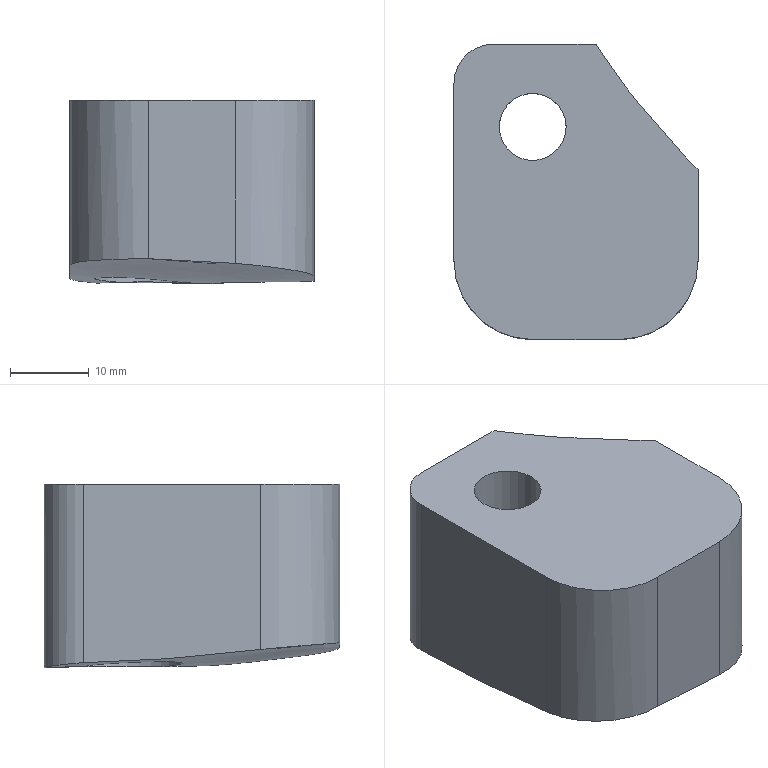Part | STEP file | gslz 2016.10.28-10_id2134_x_t | 1 solid | 16 faces | box 31 x 37.5 x 23.31 mm | volume 19794 mm3 | plane 6 | cylinder 5 | other 4 | spline 1 | commonest cylinder face diameters 20 x2 8.5 x1 10 x1 14 x1